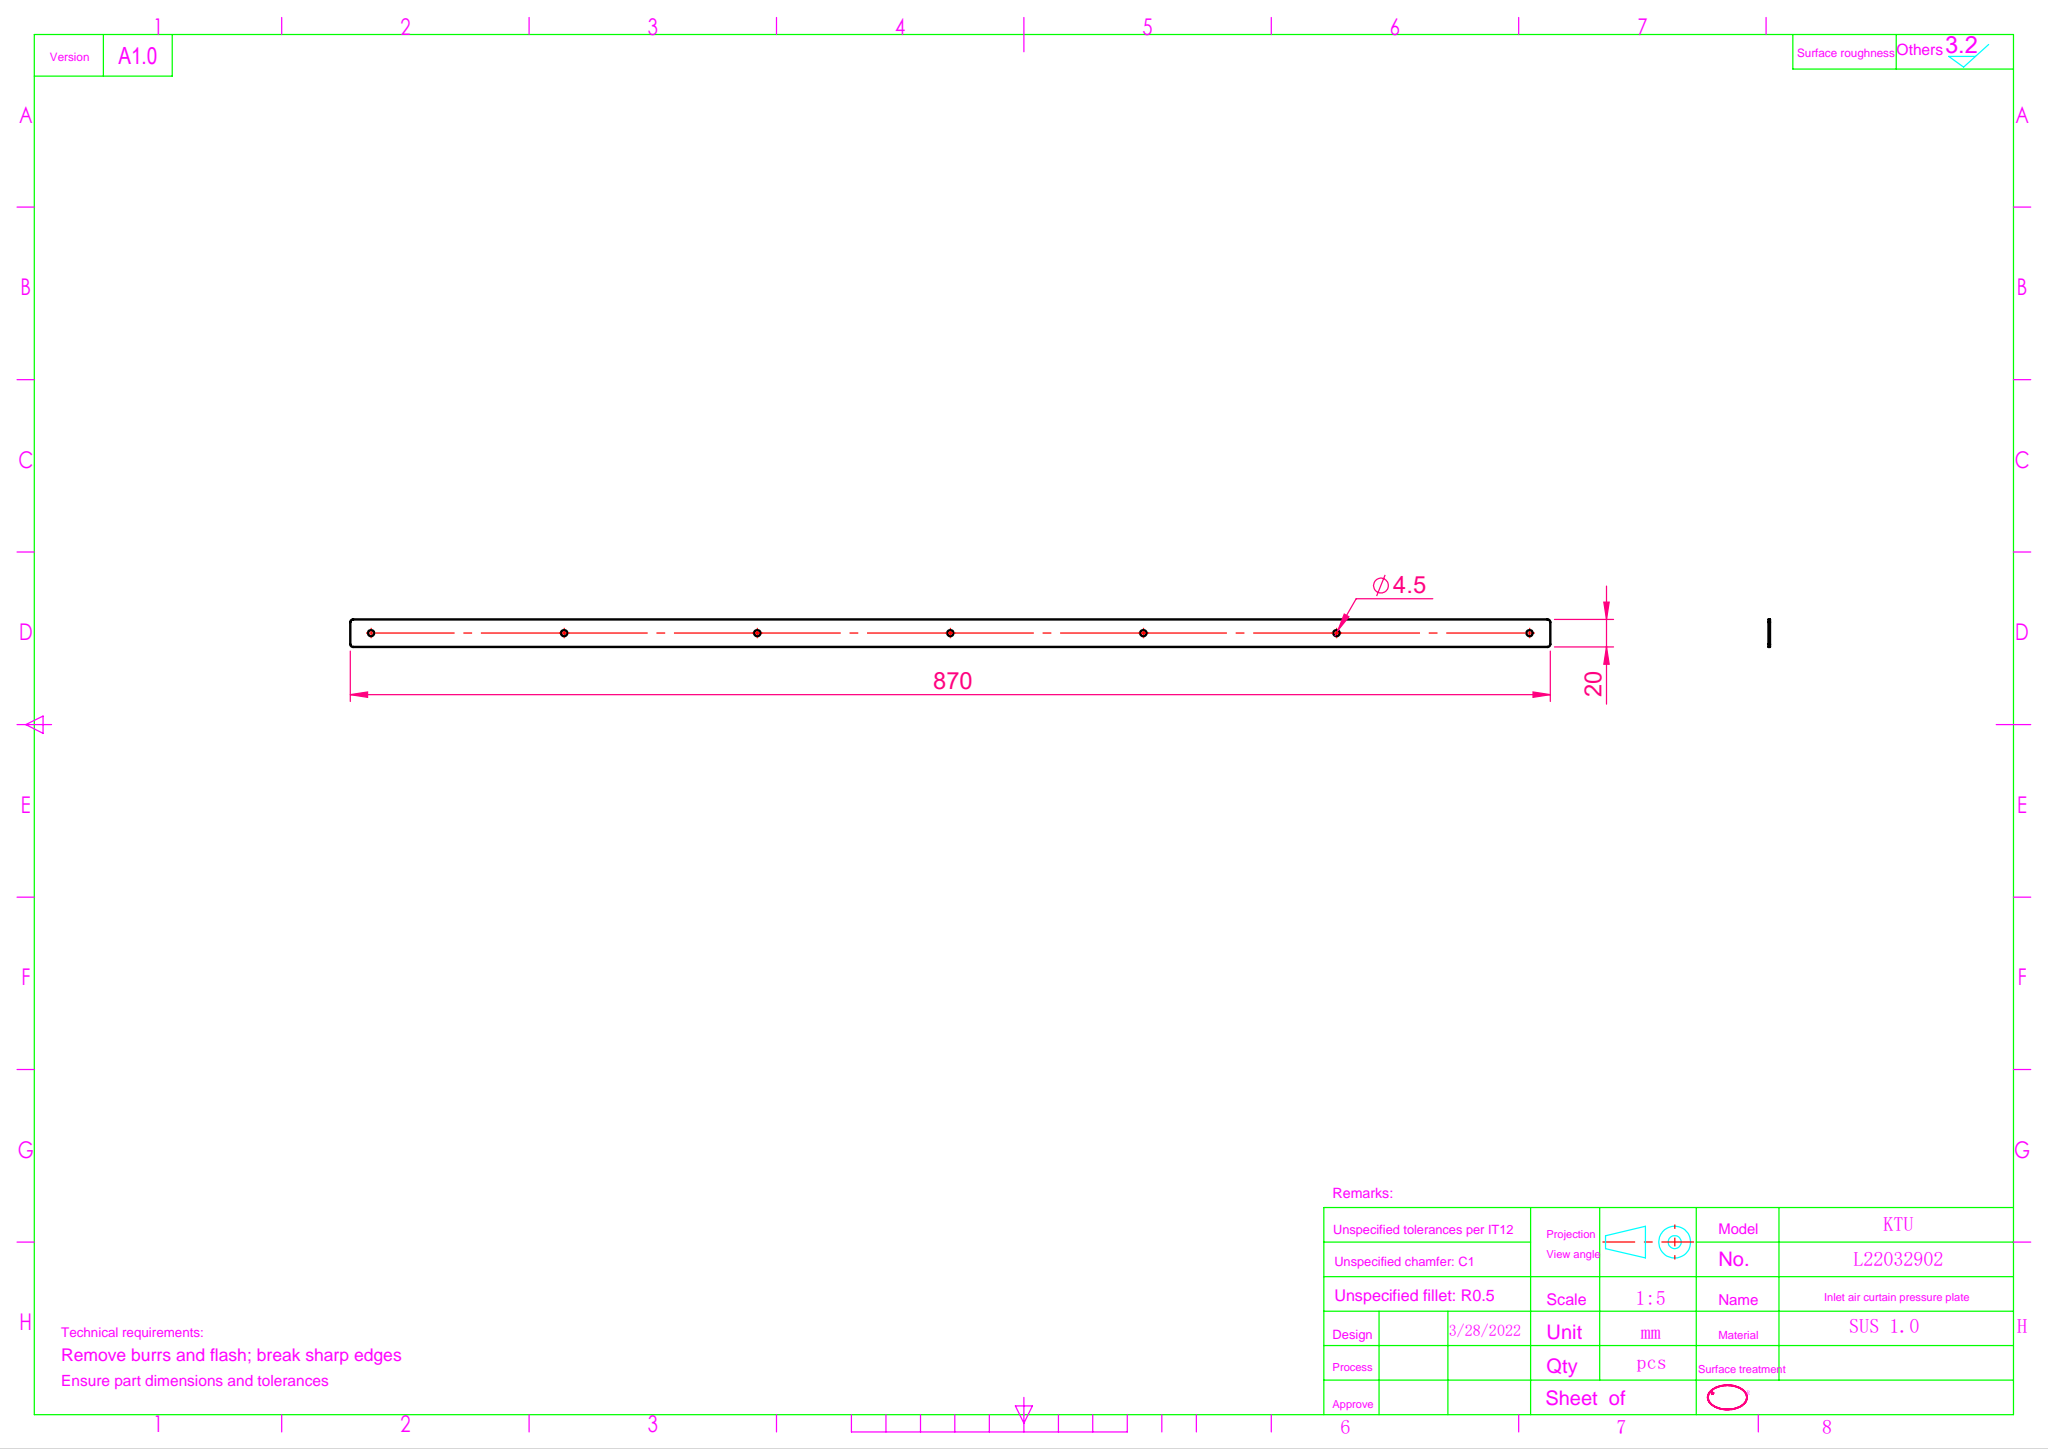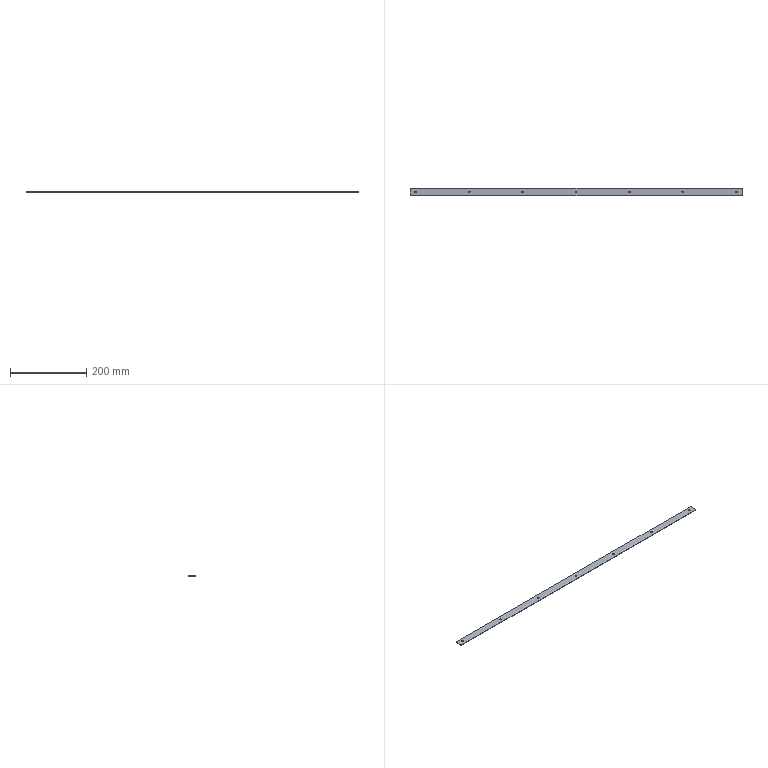Part | SolidWorks | features Fillet 1, FlatPattern 1, ICE 1, LPattern 1, SMBaseFlange 1, SheetMetal 1 | 1 solid | 24 faces | box 870 x 20 x 1 mm | volume 17285 mm3 | cylinder 18 | plane 6 | commonest cylinder face diameters 4.5 x14 4 x4
STEP:
#1=CARTESIAN_POINT('',(-282.25,0.,-1.));
#2=VERTEX_POINT('',#1);
#3=CARTESIAN_POINT('',(-277.75,0.,-1.));
#4=VERTEX_POINT('',#3);
#5=CARTESIAN_POINT('',(-280.,0.,-1.));
#6=DIRECTION('',(0.,0.,1.));
#7=DIRECTION('',(1.,0.,0.));
#8=AXIS2_PLACEMENT_3D('',#5,#6,#7);
#9=CIRCLE('',#8,2.25);
#10=EDGE_CURVE('',#2,#4,#9,.T.);
#11=ORIENTED_EDGE('',*,*,#10,.F.);
#12=CARTESIAN_POINT('',(-282.25,0.,0.));
#13=VERTEX_POINT('',#12);
#14=CARTESIAN_POINT('',(-282.25,0.,-1.));
#15=DIRECTION('',(0.,0.,1.));
#16=VECTOR('',#15,1000.);
#17=LINE('',#14,#16);
#18=EDGE_CURVE('',#2,#13,#17,.T.);
#19=ORIENTED_EDGE('',*,*,#18,.T.);
#20=CARTESIAN_POINT('',(-277.75,0.,0.));
#21=VERTEX_POINT('',#20);
#22=CARTESIAN_POINT('',(-280.,0.,0.));
#23=DIRECTION('',(0.,0.,1.));
#24=DIRECTION('',(1.,0.,0.));
#25=AXIS2_PLACEMENT_3D('',#22,#23,#24);
#26=CIRCLE('',#25,2.25);
#27=EDGE_CURVE('',#13,#21,#26,.T.);
#28=ORIENTED_EDGE('',*,*,#27,.T.);
#29=CARTESIAN_POINT('',(-277.75,0.,-1.));
#30=DIRECTION('',(0.,0.,1.));
#31=VECTOR('',#30,1000.);
#32=LINE('',#29,#31);
#33=EDGE_CURVE('',#4,#21,#32,.T.);
#34=ORIENTED_EDGE('',*,*,#33,.F.);
#35=EDGE_LOOP('',(#11,#19,#28,#34));
#36=FACE_OUTER_BOUND('',#35,.T.);
#37=CARTESIAN_POINT('',(-280.,0.,-1.));
#38=DIRECTION('',(0.,0.,1.));
#39=DIRECTION('',(1.,0.,0.));
#40=AXIS2_PLACEMENT_3D('',#37,#38,#39);
#41=CYLINDRICAL_SURFACE('',#40,2.25);
#42=ADVANCED_FACE('',(#36),#41,.F.);
#43=CARTESIAN_POINT('',(277.75,0.,-1.));
#44=VERTEX_POINT('',#43);
#45=CARTESIAN_POINT('',(282.25,0.,-1.));
#46=VERTEX_POINT('',#45);
#47=CARTESIAN_POINT('',(280.,0.,-1.));
#48=DIRECTION('',(0.,0.,1.));
#49=DIRECTION('',(1.,0.,0.));
#50=AXIS2_PLACEMENT_3D('',#47,#48,#49);
#51=CIRCLE('',#50,2.25);
#52=EDGE_CURVE('',#44,#46,#51,.T.);
#53=ORIENTED_EDGE('',*,*,#52,.F.);
#54=CARTESIAN_POINT('',(277.75,0.,0.));
#55=VERTEX_POINT('',#54);
#56=CARTESIAN_POINT('',(277.75,0.,-1.));
#57=DIRECTION('',(0.,0.,1.));
#58=VECTOR('',#57,1000.);
#59=LINE('',#56,#58);
#60=EDGE_CURVE('',#44,#55,#59,.T.);
#61=ORIENTED_EDGE('',*,*,#60,.T.);
#62=CARTESIAN_POINT('',(282.25,0.,0.));
#63=VERTEX_POINT('',#62);
#64=CARTESIAN_POINT('',(280.,0.,0.));
#65=DIRECTION('',(0.,0.,1.));
#66=DIRECTION('',(1.,0.,0.));
#67=AXIS2_PLACEMENT_3D('',#64,#65,#66);
#68=CIRCLE('',#67,2.25);
#69=EDGE_CURVE('',#55,#63,#68,.T.);
#70=ORIENTED_EDGE('',*,*,#69,.T.);
#71=CARTESIAN_POINT('',(282.25,0.,-1.));
#72=DIRECTION('',(0.,0.,1.));
#73=VECTOR('',#72,1000.);
#74=LINE('',#71,#73);
#75=EDGE_CURVE('',#46,#63,#74,.T.);
#76=ORIENTED_EDGE('',*,*,#75,.F.);
#77=EDGE_LOOP('',(#53,#61,#70,#76));
#78=FACE_OUTER_BOUND('',#77,.T.);
#79=CARTESIAN_POINT('',(280.,0.,-1.));
#80=DIRECTION('',(0.,0.,1.));
#81=DIRECTION('',(1.,0.,0.));
#82=AXIS2_PLACEMENT_3D('',#79,#80,#81);
#83=CYLINDRICAL_SURFACE('',#82,2.25);
#84=ADVANCED_FACE('',(#78),#83,.F.);
#85=CARTESIAN_POINT('',(417.75,0.,-1.));
#86=VERTEX_POINT('',#85);
#87=CARTESIAN_POINT('',(422.25,0.,-1.));
#88=VERTEX_POINT('',#87);
#89=CARTESIAN_POINT('',(420.,0.,-1.));
#90=DIRECTION('',(0.,0.,1.));
#91=DIRECTION('',(1.,0.,0.));
#92=AXIS2_PLACEMENT_3D('',#89,#90,#91);
#93=CIRCLE('',#92,2.25);
#94=EDGE_CURVE('',#86,#88,#93,.T.);
#95=ORIENTED_EDGE('',*,*,#94,.F.);
#96=CARTESIAN_POINT('',(417.75,0.,0.));
#97=VERTEX_POINT('',#96);
#98=CARTESIAN_POINT('',(417.75,0.,-1.));
#99=DIRECTION('',(0.,0.,1.));
#100=VECTOR('',#99,1000.);
#101=LINE('',#98,#100);
#102=EDGE_CURVE('',#86,#97,#101,.T.);
#103=ORIENTED_EDGE('',*,*,#102,.T.);
#104=CARTESIAN_POINT('',(422.25,0.,0.));
#105=VERTEX_POINT('',#104);
#106=CARTESIAN_POINT('',(420.,0.,0.));
#107=DIRECTION('',(0.,0.,1.));
#108=DIRECTION('',(1.,0.,0.));
#109=AXIS2_PLACEMENT_3D('',#106,#107,#108);
#110=CIRCLE('',#109,2.25);
#111=EDGE_CURVE('',#97,#105,#110,.T.);
#112=ORIENTED_EDGE('',*,*,#111,.T.);
#113=CARTESIAN_POINT('',(422.25,0.,-1.));
#114=DIRECTION('',(0.,0.,1.));
#115=VECTOR('',#114,1000.);
#116=LINE('',#113,#115);
#117=EDGE_CURVE('',#88,#105,#116,.T.);
#118=ORIENTED_EDGE('',*,*,#117,.F.);
#119=EDGE_LOOP('',(#95,#103,#112,#118));
#120=FACE_OUTER_BOUND('',#119,.T.);
#121=CARTESIAN_POINT('',(420.,0.,-1.));
#122=DIRECTION('',(0.,0.,1.));
#123=DIRECTION('',(1.,0.,0.));
#124=AXIS2_PLACEMENT_3D('',#121,#122,#123);
#125=CYLINDRICAL_SURFACE('',#124,2.25);
#126=ADVANCED_FACE('',(#120),#125,.F.);
#127=CARTESIAN_POINT('',(-142.25,0.,-1.));
#128=VERTEX_POINT('',#127);
#129=CARTESIAN_POINT('',(-137.75,0.,-1.));
#130=VERTEX_POINT('',#129);
#131=CARTESIAN_POINT('',(-140.,0.,-1.));
#132=DIRECTION('',(0.,0.,1.));
#133=DIRECTION('',(1.,0.,0.));
#134=AXIS2_PLACEMENT_3D('',#131,#132,#133);
#135=CIRCLE('',#134,2.25);
#136=EDGE_CURVE('',#128,#130,#135,.T.);
#137=ORIENTED_EDGE('',*,*,#136,.F.);
#138=CARTESIAN_POINT('',(-142.25,0.,0.));
#139=VERTEX_POINT('',#138);
#140=CARTESIAN_POINT('',(-142.25,0.,-1.));
#141=DIRECTION('',(0.,0.,1.));
#142=VECTOR('',#141,1000.);
#143=LINE('',#140,#142);
#144=EDGE_CURVE('',#128,#139,#143,.T.);
#145=ORIENTED_EDGE('',*,*,#144,.T.);
#146=CARTESIAN_POINT('',(-137.75,0.,0.));
#147=VERTEX_POINT('',#146);
#148=CARTESIAN_POINT('',(-140.,0.,0.));
#149=DIRECTION('',(0.,0.,1.));
#150=DIRECTION('',(1.,0.,0.));
#151=AXIS2_PLACEMENT_3D('',#148,#149,#150);
#152=CIRCLE('',#151,2.25);
#153=EDGE_CURVE('',#139,#147,#152,.T.);
#154=ORIENTED_EDGE('',*,*,#153,.T.);
#155=CARTESIAN_POINT('',(-137.75,0.,-1.));
#156=DIRECTION('',(0.,0.,1.));
#157=VECTOR('',#156,1000.);
#158=LINE('',#155,#157);
#159=EDGE_CURVE('',#130,#147,#158,.T.);
#160=ORIENTED_EDGE('',*,*,#159,.F.);
#161=EDGE_LOOP('',(#137,#145,#154,#160));
#162=FACE_OUTER_BOUND('',#161,.T.);
#163=CARTESIAN_POINT('',(-140.,0.,-1.));
#164=DIRECTION('',(0.,0.,1.));
#165=DIRECTION('',(1.,0.,0.));
#166=AXIS2_PLACEMENT_3D('',#163,#164,#165);
#167=CYLINDRICAL_SURFACE('',#166,2.25);
#168=ADVANCED_FACE('',(#162),#167,.F.);
#169=CARTESIAN_POINT('',(-422.25,0.,-1.));
#170=VERTEX_POINT('',#169);
#171=CARTESIAN_POINT('',(-417.75,0.,-1.));
#172=VERTEX_POINT('',#171);
#173=CARTESIAN_POINT('',(-420.,0.,-1.));
#174=DIRECTION('',(0.,0.,1.));
#175=DIRECTION('',(1.,0.,0.));
#176=AXIS2_PLACEMENT_3D('',#173,#174,#175);
#177=CIRCLE('',#176,2.25);
#178=EDGE_CURVE('',#170,#172,#177,.T.);
#179=ORIENTED_EDGE('',*,*,#178,.F.);
#180=CARTESIAN_POINT('',(-422.25,0.,0.));
#181=VERTEX_POINT('',#180);
#182=CARTESIAN_POINT('',(-422.25,0.,-1.));
#183=DIRECTION('',(0.,0.,1.));
#184=VECTOR('',#183,1000.);
#185=LINE('',#182,#184);
#186=EDGE_CURVE('',#170,#181,#185,.T.);
#187=ORIENTED_EDGE('',*,*,#186,.T.);
#188=CARTESIAN_POINT('',(-417.75,0.,0.));
#189=VERTEX_POINT('',#188);
#190=CARTESIAN_POINT('',(-420.,0.,0.));
#191=DIRECTION('',(0.,0.,1.));
#192=DIRECTION('',(1.,0.,0.));
#193=AXIS2_PLACEMENT_3D('',#190,#191,#192);
#194=CIRCLE('',#193,2.25);
#195=EDGE_CURVE('',#181,#189,#194,.T.);
#196=ORIENTED_EDGE('',*,*,#195,.T.);
#197=CARTESIAN_POINT('',(-417.75,0.,-1.));
#198=DIRECTION('',(0.,0.,1.));
#199=VECTOR('',#198,1000.);
#200=LINE('',#197,#199);
#201=EDGE_CURVE('',#172,#189,#200,.T.);
#202=ORIENTED_EDGE('',*,*,#201,.F.);
#203=EDGE_LOOP('',(#179,#187,#196,#202));
#204=FACE_OUTER_BOUND('',#203,.T.);
#205=CARTESIAN_POINT('',(-420.,0.,-1.));
#206=DIRECTION('',(0.,0.,1.));
#207=DIRECTION('',(1.,0.,0.));
#208=AXIS2_PLACEMENT_3D('',#205,#206,#207);
#209=CYLINDRICAL_SURFACE('',#208,2.25);
#210=ADVANCED_FACE('',(#204),#209,.F.);
#211=CARTESIAN_POINT('',(137.75,0.,-1.));
#212=VERTEX_POINT('',#211);
#213=CARTESIAN_POINT('',(142.25,0.,-1.));
#214=VERTEX_POINT('',#213);
#215=CARTESIAN_POINT('',(140.,0.,-1.));
#216=DIRECTION('',(0.,0.,1.));
#217=DIRECTION('',(1.,0.,0.));
#218=AXIS2_PLACEMENT_3D('',#215,#216,#217);
#219=CIRCLE('',#218,2.25);
#220=EDGE_CURVE('',#212,#214,#219,.T.);
#221=ORIENTED_EDGE('',*,*,#220,.F.);
#222=CARTESIAN_POINT('',(137.75,0.,0.));
#223=VERTEX_POINT('',#222);
#224=CARTESIAN_POINT('',(137.75,0.,-1.));
#225=DIRECTION('',(0.,0.,1.));
#226=VECTOR('',#225,1000.);
#227=LINE('',#224,#226);
#228=EDGE_CURVE('',#212,#223,#227,.T.);
#229=ORIENTED_EDGE('',*,*,#228,.T.);
#230=CARTESIAN_POINT('',(142.25,0.,0.));
#231=VERTEX_POINT('',#230);
#232=CARTESIAN_POINT('',(140.,0.,0.));
#233=DIRECTION('',(0.,0.,1.));
#234=DIRECTION('',(1.,0.,0.));
#235=AXIS2_PLACEMENT_3D('',#232,#233,#234);
#236=CIRCLE('',#235,2.25);
#237=EDGE_CURVE('',#223,#231,#236,.T.);
#238=ORIENTED_EDGE('',*,*,#237,.T.);
#239=CARTESIAN_POINT('',(142.25,0.,-1.));
#240=DIRECTION('',(0.,0.,1.));
#241=VECTOR('',#240,1000.);
#242=LINE('',#239,#241);
#243=EDGE_CURVE('',#214,#231,#242,.T.);
#244=ORIENTED_EDGE('',*,*,#243,.F.);
#245=EDGE_LOOP('',(#221,#229,#238,#244));
#246=FACE_OUTER_BOUND('',#245,.T.);
#247=CARTESIAN_POINT('',(140.,0.,-1.));
#248=DIRECTION('',(0.,0.,1.));
#249=DIRECTION('',(1.,0.,0.));
#250=AXIS2_PLACEMENT_3D('',#247,#248,#249);
#251=CYLINDRICAL_SURFACE('',#250,2.25);
#252=ADVANCED_FACE('',(#246),#251,.F.);
#253=CARTESIAN_POINT('',(-2.25,0.,-1.));
#254=VERTEX_POINT('',#253);
#255=CARTESIAN_POINT('',(2.25,0.,-1.));
#256=VERTEX_POINT('',#255);
#257=CARTESIAN_POINT('',(0.,0.,-1.));
#258=DIRECTION('',(0.,0.,1.));
#259=DIRECTION('',(1.,0.,0.));
#260=AXIS2_PLACEMENT_3D('',#257,#258,#259);
#261=CIRCLE('',#260,2.25);
#262=EDGE_CURVE('',#254,#256,#261,.T.);
#263=ORIENTED_EDGE('',*,*,#262,.F.);
#264=CARTESIAN_POINT('',(-2.25,0.,0.));
#265=VERTEX_POINT('',#264);
#266=CARTESIAN_POINT('',(-2.25,0.,-1.));
#267=DIRECTION('',(0.,0.,1.));
#268=VECTOR('',#267,1000.);
#269=LINE('',#266,#268);
#270=EDGE_CURVE('',#254,#265,#269,.T.);
#271=ORIENTED_EDGE('',*,*,#270,.T.);
#272=CARTESIAN_POINT('',(2.25,0.,0.));
#273=VERTEX_POINT('',#272);
#274=CARTESIAN_POINT('',(0.,0.,0.));
#275=DIRECTION('',(0.,0.,1.));
#276=DIRECTION('',(1.,0.,0.));
#277=AXIS2_PLACEMENT_3D('',#274,#275,#276);
#278=CIRCLE('',#277,2.25);
#279=EDGE_CURVE('',#265,#273,#278,.T.);
#280=ORIENTED_EDGE('',*,*,#279,.T.);
#281=CARTESIAN_POINT('',(2.25,0.,-1.));
#282=DIRECTION('',(0.,0.,1.));
#283=VECTOR('',#282,1000.);
#284=LINE('',#281,#283);
#285=EDGE_CURVE('',#256,#273,#284,.T.);
#286=ORIENTED_EDGE('',*,*,#285,.F.);
#287=EDGE_LOOP('',(#263,#271,#280,#286));
#288=FACE_OUTER_BOUND('',#287,.T.);
#289=CARTESIAN_POINT('',(0.,0.,-1.));
#290=DIRECTION('',(0.,0.,1.));
#291=DIRECTION('',(1.,0.,0.));
#292=AXIS2_PLACEMENT_3D('',#289,#290,#291);
#293=CYLINDRICAL_SURFACE('',#292,2.25);
#294=ADVANCED_FACE('',(#288),#293,.F.);
#295=CARTESIAN_POINT('',(435.,-8.,0.));
#296=VERTEX_POINT('',#295);
#297=CARTESIAN_POINT('',(435.,8.,0.));
#298=VERTEX_POINT('',#297);
#299=CARTESIAN_POINT('',(435.,10.,0.));
#300=DIRECTION('',(0.,1.,0.));
#301=VECTOR('',#300,1000.);
#302=LINE('',#299,#301);
#303=EDGE_CURVE('',#296,#298,#302,.T.);
#304=ORIENTED_EDGE('',*,*,#303,.F.);
#305=CARTESIAN_POINT('',(435.,-8.,-1.));
#306=VERTEX_POINT('',#305);
#307=CARTESIAN_POINT('',(435.,-8.,-1.));
#308=DIRECTION('',(0.,0.,-1.));
#309=VECTOR('',#308,1000.);
#310=LINE('',#307,#309);
#311=EDGE_CURVE('',#296,#306,#310,.T.);
#312=ORIENTED_EDGE('',*,*,#311,.T.);
#313=CARTESIAN_POINT('',(435.,8.,-1.));
#314=VERTEX_POINT('',#313);
#315=CARTESIAN_POINT('',(435.,10.,-1.));
#316=DIRECTION('',(0.,1.,0.));
#317=VECTOR('',#316,1000.);
#318=LINE('',#315,#317);
#319=EDGE_CURVE('',#306,#314,#318,.T.);
#320=ORIENTED_EDGE('',*,*,#319,.T.);
#321=CARTESIAN_POINT('',(435.,8.,-1.));
#322=DIRECTION('',(0.,0.,1.));
#323=VECTOR('',#322,1000.);
#324=LINE('',#321,#323);
#325=EDGE_CURVE('',#314,#298,#324,.T.);
#326=ORIENTED_EDGE('',*,*,#325,.T.);
#327=EDGE_LOOP('',(#304,#312,#320,#326));
#328=FACE_OUTER_BOUND('',#327,.T.);
#329=CARTESIAN_POINT('',(435.,10.,-1.));
#330=DIRECTION('',(1.,0.,0.));
#331=DIRECTION('',(0.,0.,-1.));
#332=AXIS2_PLACEMENT_3D('',#329,#330,#331);
#333=PLANE('',#332);
#334=ADVANCED_FACE('',(#328),#333,.T.);
#335=CARTESIAN_POINT('',(-433.,-10.,-1.));
#336=VERTEX_POINT('',#335);
#337=CARTESIAN_POINT('',(433.,-10.,-1.));
#338=VERTEX_POINT('',#337);
#339=CARTESIAN_POINT('',(-435.,-10.,-1.));
#340=DIRECTION('',(1.,0.,0.));
#341=VECTOR('',#340,1000.);
#342=LINE('',#339,#341);
#343=EDGE_CURVE('',#336,#338,#342,.T.);
#344=ORIENTED_EDGE('',*,*,#343,.T.);
#345=CARTESIAN_POINT('',(433.,-10.,0.));
#346=VERTEX_POINT('',#345);
#347=CARTESIAN_POINT('',(433.,-10.,-1.));
#348=DIRECTION('',(0.,0.,1.));
#349=VECTOR('',#348,1000.);
#350=LINE('',#347,#349);
#351=EDGE_CURVE('',#338,#346,#350,.T.);
#352=ORIENTED_EDGE('',*,*,#351,.T.);
#353=CARTESIAN_POINT('',(-433.,-10.,0.));
#354=VERTEX_POINT('',#353);
#355=CARTESIAN_POINT('',(-435.,-10.,0.));
#356=DIRECTION('',(1.,0.,0.));
#357=VECTOR('',#356,1000.);
#358=LINE('',#355,#357);
#359=EDGE_CURVE('',#354,#346,#358,.T.);
#360=ORIENTED_EDGE('',*,*,#359,.F.);
#361=CARTESIAN_POINT('',(-433.,-10.,-1.));
#362=DIRECTION('',(0.,0.,-1.));
#363=VECTOR('',#362,1000.);
#364=LINE('',#361,#363);
#365=EDGE_CURVE('',#354,#336,#364,.T.);
#366=ORIENTED_EDGE('',*,*,#365,.T.);
#367=EDGE_LOOP('',(#344,#352,#360,#366));
#368=FACE_OUTER_BOUND('',#367,.T.);
#369=CARTESIAN_POINT('',(-435.,-10.,-1.));
#370=DIRECTION('',(0.,-1.,0.));
#371=DIRECTION('',(0.,0.,-1.));
#372=AXIS2_PLACEMENT_3D('',#369,#370,#371);
#373=PLANE('',#372);
#374=ADVANCED_FACE('',(#368),#373,.T.);
#375=CARTESIAN_POINT('',(-435.,8.,-1.));
#376=VERTEX_POINT('',#375);
#377=CARTESIAN_POINT('',(-435.,-8.,-1.));
#378=VERTEX_POINT('',#377);
#379=CARTESIAN_POINT('',(-435.,10.,-1.));
#380=DIRECTION('',(0.,-1.,0.));
#381=VECTOR('',#380,1000.);
#382=LINE('',#379,#381);
#383=EDGE_CURVE('',#376,#378,#382,.T.);
#384=ORIENTED_EDGE('',*,*,#383,.T.);
#385=CARTESIAN_POINT('',(-435.,-8.,0.));
#386=VERTEX_POINT('',#385);
#387=CARTESIAN_POINT('',(-435.,-8.,-1.));
#388=DIRECTION('',(0.,0.,1.));
#389=VECTOR('',#388,1000.);
#390=LINE('',#387,#389);
#391=EDGE_CURVE('',#378,#386,#390,.T.);
#392=ORIENTED_EDGE('',*,*,#391,.T.);
#393=CARTESIAN_POINT('',(-435.,8.,0.));
#394=VERTEX_POINT('',#393);
#395=CARTESIAN_POINT('',(-435.,10.,0.));
#396=DIRECTION('',(0.,-1.,0.));
#397=VECTOR('',#396,1000.);
#398=LINE('',#395,#397);
#399=EDGE_CURVE('',#394,#386,#398,.T.);
#400=ORIENTED_EDGE('',*,*,#399,.F.);
#401=CARTESIAN_POINT('',(-435.,8.,-1.));
#402=DIRECTION('',(0.,0.,-1.));
#403=VECTOR('',#402,1000.);
#404=LINE('',#401,#403);
#405=EDGE_CURVE('',#394,#376,#404,.T.);
#406=ORIENTED_EDGE('',*,*,#405,.T.);
#407=EDGE_LOOP('',(#384,#392,#400,#406));
#408=FACE_OUTER_BOUND('',#407,.T.);
#409=CARTESIAN_POINT('',(-435.,10.,-1.));
#410=DIRECTION('',(-1.,0.,0.));
#411=DIRECTION('',(0.,0.,1.));
#412=AXIS2_PLACEMENT_3D('',#409,#410,#411);
#413=PLANE('',#412);
#414=ADVANCED_FACE('',(#408),#413,.T.);
#415=CARTESIAN_POINT('',(433.,10.,0.));
#416=VERTEX_POINT('',#415);
#417=CARTESIAN_POINT('',(-433.,10.,0.));
#418=VERTEX_POINT('',#417);
#419=CARTESIAN_POINT('',(-435.,10.,0.));
#420=DIRECTION('',(-1.,0.,0.));
#421=VECTOR('',#420,1000.);
#422=LINE('',#419,#421);
#423=EDGE_CURVE('',#416,#418,#422,.T.);
#424=ORIENTED_EDGE('',*,*,#423,.F.);
#425=CARTESIAN_POINT('',(433.,10.,-1.));
#426=VERTEX_POINT('',#425);
#427=CARTESIAN_POINT('',(433.,10.,-1.));
#428=DIRECTION('',(0.,0.,-1.));
#429=VECTOR('',#428,1000.);
#430=LINE('',#427,#429);
#431=EDGE_CURVE('',#416,#426,#430,.T.);
#432=ORIENTED_EDGE('',*,*,#431,.T.);
#433=CARTESIAN_POINT('',(-433.,10.,-1.));
#434=VERTEX_POINT('',#433);
#435=CARTESIAN_POINT('',(-435.,10.,-1.));
#436=DIRECTION('',(-1.,0.,0.));
#437=VECTOR('',#436,1000.);
#438=LINE('',#435,#437);
#439=EDGE_CURVE('',#426,#434,#438,.T.);
#440=ORIENTED_EDGE('',*,*,#439,.T.);
#441=CARTESIAN_POINT('',(-433.,10.,-1.));
#442=DIRECTION('',(0.,0.,1.));
#443=VECTOR('',#442,1000.);
#444=LINE('',#441,#443);
#445=EDGE_CURVE('',#434,#418,#444,.T.);
#446=ORIENTED_EDGE('',*,*,#445,.T.);
#447=EDGE_LOOP('',(#424,#432,#440,#446));
#448=FACE_OUTER_BOUND('',#447,.T.);
#449=CARTESIAN_POINT('',(-435.,10.,-1.));
#450=DIRECTION('',(0.,1.,0.));
#451=DIRECTION('',(0.,0.,1.));
#452=AXIS2_PLACEMENT_3D('',#449,#450,#451);
#453=PLANE('',#452);
#454=ADVANCED_FACE('',(#448),#453,.T.);
#455=CARTESIAN_POINT('',(-280.,0.,-1.));
#456=DIRECTION('',(0.,0.,1.));
#457=DIRECTION('',(1.,0.,0.));
#458=AXIS2_PLACEMENT_3D('',#455,#456,#457);
#459=CIRCLE('',#458,2.25);
#460=EDGE_CURVE('',#4,#2,#459,.T.);
#461=ORIENTED_EDGE('',*,*,#460,.T.);
#462=ORIENTED_EDGE('',*,*,#10,.T.);
#463=EDGE_LOOP('',(#461,#462));
#464=FACE_BOUND('',#463,.T.);
#465=CARTESIAN_POINT('',(280.,0.,-1.));
#466=DIRECTION('',(0.,0.,1.));
#467=DIRECTION('',(1.,0.,0.));
#468=AXIS2_PLACEMENT_3D('',#465,#466,#467);
#469=CIRCLE('',#468,2.25);
#470=EDGE_CURVE('',#46,#44,#469,.T.);
#471=ORIENTED_EDGE('',*,*,#470,.T.);
#472=ORIENTED_EDGE('',*,*,#52,.T.);
#473=EDGE_LOOP('',(#471,#472));
#474=FACE_BOUND('',#473,.T.);
#475=CARTESIAN_POINT('',(420.,0.,-1.));
#476=DIRECTION('',(0.,0.,1.));
#477=DIRECTION('',(1.,0.,0.));
#478=AXIS2_PLACEMENT_3D('',#475,#476,#477);
#479=CIRCLE('',#478,2.25);
#480=EDGE_CURVE('',#88,#86,#479,.T.);
#481=ORIENTED_EDGE('',*,*,#480,.T.);
#482=ORIENTED_EDGE('',*,*,#94,.T.);
#483=EDGE_LOOP('',(#481,#482));
#484=FACE_BOUND('',#483,.T.);
#485=CARTESIAN_POINT('',(-140.,0.,-1.));
#486=DIRECTION('',(0.,0.,1.));
#487=DIRECTION('',(1.,0.,0.));
#488=AXIS2_PLACEMENT_3D('',#485,#486,#487);
#489=CIRCLE('',#488,2.25);
#490=EDGE_CURVE('',#130,#128,#489,.T.);
#491=ORIENTED_EDGE('',*,*,#490,.T.);
#492=ORIENTED_EDGE('',*,*,#136,.T.);
#493=EDGE_LOOP('',(#491,#492));
#494=FACE_BOUND('',#493,.T.);
#495=CARTESIAN_POINT('',(-420.,0.,-1.));
#496=DIRECTION('',(0.,0.,1.));
#497=DIRECTION('',(1.,0.,0.));
#498=AXIS2_PLACEMENT_3D('',#495,#496,#497);
#499=CIRCLE('',#498,2.25);
#500=EDGE_CURVE('',#172,#170,#499,.T.);
#501=ORIENTED_EDGE('',*,*,#500,.T.);
#502=ORIENTED_EDGE('',*,*,#178,.T.);
#503=EDGE_LOOP('',(#501,#502));
#504=FACE_BOUND('',#503,.T.);
#505=CARTESIAN_POINT('',(140.,0.,-1.));
#506=DIRECTION('',(0.,0.,1.));
#507=DIRECTION('',(1.,0.,0.));
#508=AXIS2_PLACEMENT_3D('',#505,#506,#507);
#509=CIRCLE('',#508,2.25);
#510=EDGE_CURVE('',#214,#212,#509,.T.);
#511=ORIENTED_EDGE('',*,*,#510,.T.);
#512=ORIENTED_EDGE('',*,*,#220,.T.);
#513=EDGE_LOOP('',(#511,#512));
#514=FACE_BOUND('',#513,.T.);
#515=CARTESIAN_POINT('',(0.,0.,-1.));
#516=DIRECTION('',(0.,0.,1.));
#517=DIRECTION('',(1.,0.,0.));
#518=AXIS2_PLACEMENT_3D('',#515,#516,#517);
#519=CIRCLE('',#518,2.25);
#520=EDGE_CURVE('',#256,#254,#519,.T.);
#521=ORIENTED_EDGE('',*,*,#520,.T.);
#522=ORIENTED_EDGE('',*,*,#262,.T.);
#523=EDGE_LOOP('',(#521,#522));
#524=FACE_BOUND('',#523,.T.);
#525=ORIENTED_EDGE('',*,*,#319,.F.);
#526=CARTESIAN_POINT('',(433.,-8.,-1.));
#527=DIRECTION('',(0.,0.,-1.));
#528=DIRECTION('',(1.,0.,0.));
#529=AXIS2_PLACEMENT_3D('',#526,#527,#528);
#530=CIRCLE('',#529,2.);
#531=EDGE_CURVE('',#306,#338,#530,.T.);
#532=ORIENTED_EDGE('',*,*,#531,.T.);
#533=ORIENTED_EDGE('',*,*,#343,.F.);
#534=CARTESIAN_POINT('',(-433.,-8.,-1.));
#535=DIRECTION('',(0.,0.,-1.));
#536=DIRECTION('',(1.,0.,0.));
#537=AXIS2_PLACEMENT_3D('',#534,#535,#536);
#538=CIRCLE('',#537,2.);
#539=EDGE_CURVE('',#336,#378,#538,.T.);
#540=ORIENTED_EDGE('',*,*,#539,.T.);
#541=ORIENTED_EDGE('',*,*,#383,.F.);
#542=CARTESIAN_POINT('',(-433.,8.,-1.));
#543=DIRECTION('',(0.,0.,-1.));
#544=DIRECTION('',(1.,0.,0.));
#545=AXIS2_PLACEMENT_3D('',#542,#543,#544);
#546=CIRCLE('',#545,2.);
#547=EDGE_CURVE('',#376,#434,#546,.T.);
#548=ORIENTED_EDGE('',*,*,#547,.T.);
#549=ORIENTED_EDGE('',*,*,#439,.F.);
#550=CARTESIAN_POINT('',(433.,8.,-1.));
#551=DIRECTION('',(0.,0.,-1.));
#552=DIRECTION('',(1.,0.,0.));
#553=AXIS2_PLACEMENT_3D('',#550,#551,#552);
#554=CIRCLE('',#553,2.);
#555=EDGE_CURVE('',#426,#314,#554,.T.);
#556=ORIENTED_EDGE('',*,*,#555,.T.);
#557=EDGE_LOOP('',(#525,#532,#533,#540,#541,#548,#549,#556));
#558=FACE_OUTER_BOUND('',#557,.T.);
#559=CARTESIAN_POINT('',(0.,0.,-1.));
#560=DIRECTION('',(0.,0.,1.));
#561=DIRECTION('',(1.,0.,0.));
#562=AXIS2_PLACEMENT_3D('',#559,#560,#561);
#563=PLANE('',#562);
#564=ADVANCED_FACE('',(#464,#474,#484,#494,#504,#514,#524,#558),#563,.F.);
#565=CARTESIAN_POINT('',(-280.,0.,0.));
#566=DIRECTION('',(0.,0.,1.));
#567=DIRECTION('',(1.,0.,0.));
#568=AXIS2_PLACEMENT_3D('',#565,#566,#567);
#569=CIRCLE('',#568,2.25);
#570=EDGE_CURVE('',#21,#13,#569,.T.);
#571=ORIENTED_EDGE('',*,*,#570,.F.);
#572=ORIENTED_EDGE('',*,*,#27,.F.);
#573=EDGE_LOOP('',(#571,#572));
#574=FACE_BOUND('',#573,.T.);
#575=CARTESIAN_POINT('',(280.,0.,0.));
#576=DIRECTION('',(0.,0.,1.));
#577=DIRECTION('',(1.,0.,0.));
#578=AXIS2_PLACEMENT_3D('',#575,#576,#577);
#579=CIRCLE('',#578,2.25);
#580=EDGE_CURVE('',#63,#55,#579,.T.);
#581=ORIENTED_EDGE('',*,*,#580,.F.);
#582=ORIENTED_EDGE('',*,*,#69,.F.);
#583=EDGE_LOOP('',(#581,#582));
#584=FACE_BOUND('',#583,.T.);
#585=CARTESIAN_POINT('',(420.,0.,0.));
#586=DIRECTION('',(0.,0.,1.));
#587=DIRECTION('',(1.,0.,0.));
#588=AXIS2_PLACEMENT_3D('',#585,#586,#587);
#589=CIRCLE('',#588,2.25);
#590=EDGE_CURVE('',#105,#97,#589,.T.);
#591=ORIENTED_EDGE('',*,*,#590,.F.);
#592=ORIENTED_EDGE('',*,*,#111,.F.);
#593=EDGE_LOOP('',(#591,#592));
#594=FACE_BOUND('',#593,.T.);
#595=CARTESIAN_POINT('',(-140.,0.,0.));
#596=DIRECTION('',(0.,0.,1.));
#597=DIRECTION('',(1.,0.,0.));
#598=AXIS2_PLACEMENT_3D('',#595,#596,#597);
#599=CIRCLE('',#598,2.25);
#600=EDGE_CURVE('',#147,#139,#599,.T.);
#601=ORIENTED_EDGE('',*,*,#600,.F.);
#602=ORIENTED_EDGE('',*,*,#153,.F.);
#603=EDGE_LOOP('',(#601,#602));
#604=FACE_BOUND('',#603,.T.);
#605=CARTESIAN_POINT('',(-420.,0.,0.));
#606=DIRECTION('',(0.,0.,1.));
#607=DIRECTION('',(1.,0.,0.));
#608=AXIS2_PLACEMENT_3D('',#605,#606,#607);
#609=CIRCLE('',#608,2.25);
#610=EDGE_CURVE('',#189,#181,#609,.T.);
#611=ORIENTED_EDGE('',*,*,#610,.F.);
#612=ORIENTED_EDGE('',*,*,#195,.F.);
#613=EDGE_LOOP('',(#611,#612));
#614=FACE_BOUND('',#613,.T.);
#615=CARTESIAN_POINT('',(140.,0.,0.));
#616=DIRECTION('',(0.,0.,1.));
#617=DIRECTION('',(1.,0.,0.));
#618=AXIS2_PLACEMENT_3D('',#615,#616,#617);
#619=CIRCLE('',#618,2.25);
#620=EDGE_CURVE('',#231,#223,#619,.T.);
#621=ORIENTED_EDGE('',*,*,#620,.F.);
#622=ORIENTED_EDGE('',*,*,#237,.F.);
#623=EDGE_LOOP('',(#621,#622));
#624=FACE_BOUND('',#623,.T.);
#625=CARTESIAN_POINT('',(0.,0.,0.));
#626=DIRECTION('',(0.,0.,1.));
#627=DIRECTION('',(1.,0.,0.));
#628=AXIS2_PLACEMENT_3D('',#625,#626,#627);
#629=CIRCLE('',#628,2.25);
#630=EDGE_CURVE('',#273,#265,#629,.T.);
#631=ORIENTED_EDGE('',*,*,#630,.F.);
#632=ORIENTED_EDGE('',*,*,#279,.F.);
#633=EDGE_LOOP('',(#631,#632));
#634=FACE_BOUND('',#633,.T.);
#635=ORIENTED_EDGE('',*,*,#359,.T.);
#636=CARTESIAN_POINT('',(433.,-8.,0.));
#637=DIRECTION('',(0.,0.,1.));
#638=DIRECTION('',(1.,0.,0.));
#639=AXIS2_PLACEMENT_3D('',#636,#637,#638);
#640=CIRCLE('',#639,2.);
#641=EDGE_CURVE('',#346,#296,#640,.T.);
#642=ORIENTED_EDGE('',*,*,#641,.T.);
#643=ORIENTED_EDGE('',*,*,#303,.T.);
#644=CARTESIAN_POINT('',(433.,8.,0.));
#645=DIRECTION('',(0.,0.,1.));
#646=DIRECTION('',(1.,0.,0.));
#647=AXIS2_PLACEMENT_3D('',#644,#645,#646);
#648=CIRCLE('',#647,2.);
#649=EDGE_CURVE('',#298,#416,#648,.T.);
#650=ORIENTED_EDGE('',*,*,#649,.T.);
#651=ORIENTED_EDGE('',*,*,#423,.T.);
#652=CARTESIAN_POINT('',(-433.,8.,0.));
#653=DIRECTION('',(0.,0.,1.));
#654=DIRECTION('',(1.,0.,0.));
#655=AXIS2_PLACEMENT_3D('',#652,#653,#654);
#656=CIRCLE('',#655,2.);
#657=EDGE_CURVE('',#418,#394,#656,.T.);
#658=ORIENTED_EDGE('',*,*,#657,.T.);
#659=ORIENTED_EDGE('',*,*,#399,.T.);
#660=CARTESIAN_POINT('',(-433.,-8.,0.));
#661=DIRECTION('',(0.,0.,1.));
#662=DIRECTION('',(1.,0.,0.));
#663=AXIS2_PLACEMENT_3D('',#660,#661,#662);
#664=CIRCLE('',#663,2.);
#665=EDGE_CURVE('',#386,#354,#664,.T.);
#666=ORIENTED_EDGE('',*,*,#665,.T.);
#667=EDGE_LOOP('',(#635,#642,#643,#650,#651,#658,#659,#666));
#668=FACE_OUTER_BOUND('',#667,.T.);
#669=CARTESIAN_POINT('',(0.,0.,0.));
#670=DIRECTION('',(0.,0.,1.));
#671=DIRECTION('',(1.,0.,0.));
#672=AXIS2_PLACEMENT_3D('',#669,#670,#671);
#673=PLANE('',#672);
#674=ADVANCED_FACE('',(#574,#584,#594,#604,#614,#624,#634,#668),#673,.T.);
#675=ORIENTED_EDGE('',*,*,#270,.F.);
#676=ORIENTED_EDGE('',*,*,#520,.F.);
#677=ORIENTED_EDGE('',*,*,#285,.T.);
#678=ORIENTED_EDGE('',*,*,#630,.T.);
#679=EDGE_LOOP('',(#675,#676,#677,#678));
#680=FACE_OUTER_BOUND('',#679,.T.);
#681=CARTESIAN_POINT('',(0.,0.,-1.));
#682=DIRECTION('',(0.,0.,1.));
#683=DIRECTION('',(1.,0.,0.));
#684=AXIS2_PLACEMENT_3D('',#681,#682,#683);
#685=CYLINDRICAL_SURFACE('',#684,2.25);
#686=ADVANCED_FACE('',(#680),#685,.F.);
#687=ORIENTED_EDGE('',*,*,#228,.F.);
#688=ORIENTED_EDGE('',*,*,#510,.F.);
#689=ORIENTED_EDGE('',*,*,#243,.T.);
#690=ORIENTED_EDGE('',*,*,#620,.T.);
#691=EDGE_LOOP('',(#687,#688,#689,#690));
#692=FACE_OUTER_BOUND('',#691,.T.);
#693=CARTESIAN_POINT('',(140.,0.,-1.));
#694=DIRECTION('',(0.,0.,1.));
#695=DIRECTION('',(1.,0.,0.));
#696=AXIS2_PLACEMENT_3D('',#693,#694,#695);
#697=CYLINDRICAL_SURFACE('',#696,2.25);
#698=ADVANCED_FACE('',(#692),#697,.F.);
#699=ORIENTED_EDGE('',*,*,#186,.F.);
#700=ORIENTED_EDGE('',*,*,#500,.F.);
#701=ORIENTED_EDGE('',*,*,#201,.T.);
#702=ORIENTED_EDGE('',*,*,#610,.T.);
#703=EDGE_LOOP('',(#699,#700,#701,#702));
#704=FACE_OUTER_BOUND('',#703,.T.);
#705=CARTESIAN_POINT('',(-420.,0.,-1.));
#706=DIRECTION('',(0.,0.,1.));
#707=DIRECTION('',(1.,0.,0.));
#708=AXIS2_PLACEMENT_3D('',#705,#706,#707);
#709=CYLINDRICAL_SURFACE('',#708,2.25);
#710=ADVANCED_FACE('',(#704),#709,.F.);
#711=ORIENTED_EDGE('',*,*,#144,.F.);
#712=ORIENTED_EDGE('',*,*,#490,.F.);
#713=ORIENTED_EDGE('',*,*,#159,.T.);
#714=ORIENTED_EDGE('',*,*,#600,.T.);
#715=EDGE_LOOP('',(#711,#712,#713,#714));
#716=FACE_OUTER_BOUND('',#715,.T.);
#717=CARTESIAN_POINT('',(-140.,0.,-1.));
#718=DIRECTION('',(0.,0.,1.));
#719=DIRECTION('',(1.,0.,0.));
#720=AXIS2_PLACEMENT_3D('',#717,#718,#719);
#721=CYLINDRICAL_SURFACE('',#720,2.25);
#722=ADVANCED_FACE('',(#716),#721,.F.);
#723=ORIENTED_EDGE('',*,*,#102,.F.);
#724=ORIENTED_EDGE('',*,*,#480,.F.);
#725=ORIENTED_EDGE('',*,*,#117,.T.);
#726=ORIENTED_EDGE('',*,*,#590,.T.);
#727=EDGE_LOOP('',(#723,#724,#725,#726));
#728=FACE_OUTER_BOUND('',#727,.T.);
#729=CARTESIAN_POINT('',(420.,0.,-1.));
#730=DIRECTION('',(0.,0.,1.));
#731=DIRECTION('',(1.,0.,0.));
#732=AXIS2_PLACEMENT_3D('',#729,#730,#731);
#733=CYLINDRICAL_SURFACE('',#732,2.25);
#734=ADVANCED_FACE('',(#728),#733,.F.);
#735=ORIENTED_EDGE('',*,*,#60,.F.);
#736=ORIENTED_EDGE('',*,*,#470,.F.);
#737=ORIENTED_EDGE('',*,*,#75,.T.);
#738=ORIENTED_EDGE('',*,*,#580,.T.);
#739=EDGE_LOOP('',(#735,#736,#737,#738));
#740=FACE_OUTER_BOUND('',#739,.T.);
#741=CARTESIAN_POINT('',(280.,0.,-1.));
#742=DIRECTION('',(0.,0.,1.));
#743=DIRECTION('',(1.,0.,0.));
#744=AXIS2_PLACEMENT_3D('',#741,#742,#743);
#745=CYLINDRICAL_SURFACE('',#744,2.25);
#746=ADVANCED_FACE('',(#740),#745,.F.);
#747=ORIENTED_EDGE('',*,*,#18,.F.);
#748=ORIENTED_EDGE('',*,*,#460,.F.);
#749=ORIENTED_EDGE('',*,*,#33,.T.);
#750=ORIENTED_EDGE('',*,*,#570,.T.);
#751=EDGE_LOOP('',(#747,#748,#749,#750));
#752=FACE_OUTER_BOUND('',#751,.T.);
#753=CARTESIAN_POINT('',(-280.,0.,-1.));
#754=DIRECTION('',(0.,0.,1.));
#755=DIRECTION('',(1.,0.,0.));
#756=AXIS2_PLACEMENT_3D('',#753,#754,#755);
#757=CYLINDRICAL_SURFACE('',#756,2.25);
#758=ADVANCED_FACE('',(#752),#757,.F.);
#759=ORIENTED_EDGE('',*,*,#531,.F.);
#760=ORIENTED_EDGE('',*,*,#311,.F.);
#761=ORIENTED_EDGE('',*,*,#641,.F.);
#762=ORIENTED_EDGE('',*,*,#351,.F.);
#763=EDGE_LOOP('',(#759,#760,#761,#762));
#764=FACE_OUTER_BOUND('',#763,.T.);
#765=CARTESIAN_POINT('',(433.,-8.,-1.));
#766=DIRECTION('',(0.,0.,1.));
#767=DIRECTION('',(1.,0.,0.));
#768=AXIS2_PLACEMENT_3D('',#765,#766,#767);
#769=CYLINDRICAL_SURFACE('',#768,2.);
#770=ADVANCED_FACE('',(#764),#769,.T.);
#771=ORIENTED_EDGE('',*,*,#555,.F.);
#772=ORIENTED_EDGE('',*,*,#431,.F.);
#773=ORIENTED_EDGE('',*,*,#649,.F.);
#774=ORIENTED_EDGE('',*,*,#325,.F.);
#775=EDGE_LOOP('',(#771,#772,#773,#774));
#776=FACE_OUTER_BOUND('',#775,.T.);
#777=CARTESIAN_POINT('',(433.,8.,-1.));
#778=DIRECTION('',(0.,0.,1.));
#779=DIRECTION('',(1.,0.,0.));
#780=AXIS2_PLACEMENT_3D('',#777,#778,#779);
#781=CYLINDRICAL_SURFACE('',#780,2.);
#782=ADVANCED_FACE('',(#776),#781,.T.);
#783=ORIENTED_EDGE('',*,*,#539,.F.);
#784=ORIENTED_EDGE('',*,*,#365,.F.);
#785=ORIENTED_EDGE('',*,*,#665,.F.);
#786=ORIENTED_EDGE('',*,*,#391,.F.);
#787=EDGE_LOOP('',(#783,#784,#785,#786));
#788=FACE_OUTER_BOUND('',#787,.T.);
#789=CARTESIAN_POINT('',(-433.,-8.,-1.));
#790=DIRECTION('',(0.,0.,1.));
#791=DIRECTION('',(1.,0.,0.));
#792=AXIS2_PLACEMENT_3D('',#789,#790,#791);
#793=CYLINDRICAL_SURFACE('',#792,2.);
#794=ADVANCED_FACE('',(#788),#793,.T.);
#795=ORIENTED_EDGE('',*,*,#547,.F.);
#796=ORIENTED_EDGE('',*,*,#405,.F.);
#797=ORIENTED_EDGE('',*,*,#657,.F.);
#798=ORIENTED_EDGE('',*,*,#445,.F.);
#799=EDGE_LOOP('',(#795,#796,#797,#798));
#800=FACE_OUTER_BOUND('',#799,.T.);
#801=CARTESIAN_POINT('',(-433.,8.,-1.));
#802=DIRECTION('',(0.,0.,1.));
#803=DIRECTION('',(1.,0.,0.));
#804=AXIS2_PLACEMENT_3D('',#801,#802,#803);
#805=CYLINDRICAL_SURFACE('',#804,2.);
#806=ADVANCED_FACE('',(#800),#805,.T.);
#807=CLOSED_SHELL('',(#42,#84,#126,#168,#210,#252,#294,#334,#374,#414,#454,#564,#674,#686,#698,#710,#722,#734,#746,#758,#770,#782,#794,#806));
#808=MANIFOLD_SOLID_BREP('',#807);
#809=CARTESIAN_POINT('',(0.,0.,0.));
#810=DIRECTION('',(0.,0.,1.));
#811=DIRECTION('',(1.,0.,0.));
#812=AXIS2_PLACEMENT_3D('',#809,#810,#811);
#813=(LENGTH_UNIT()NAMED_UNIT(*)SI_UNIT(.MILLI.,.METRE.));
#814=UNCERTAINTY_MEASURE_WITH_UNIT(LENGTH_MEASURE(0.00001),#813,'','');
#815=(NAMED_UNIT(*)PLANE_ANGLE_UNIT()SI_UNIT($,.RADIAN.));
#816=(NAMED_UNIT(*)SI_UNIT($,.STERADIAN.)SOLID_ANGLE_UNIT());
#817=(GEOMETRIC_REPRESENTATION_CONTEXT(3)GLOBAL_UNCERTAINTY_ASSIGNED_CONTEXT((#814))GLOBAL_UNIT_ASSIGNED_CONTEXT((#813,#815,#816))REPRESENTATION_CONTEXT('',''));
#818=ADVANCED_BREP_SHAPE_REPRESENTATION('',(#808,#812),#817);